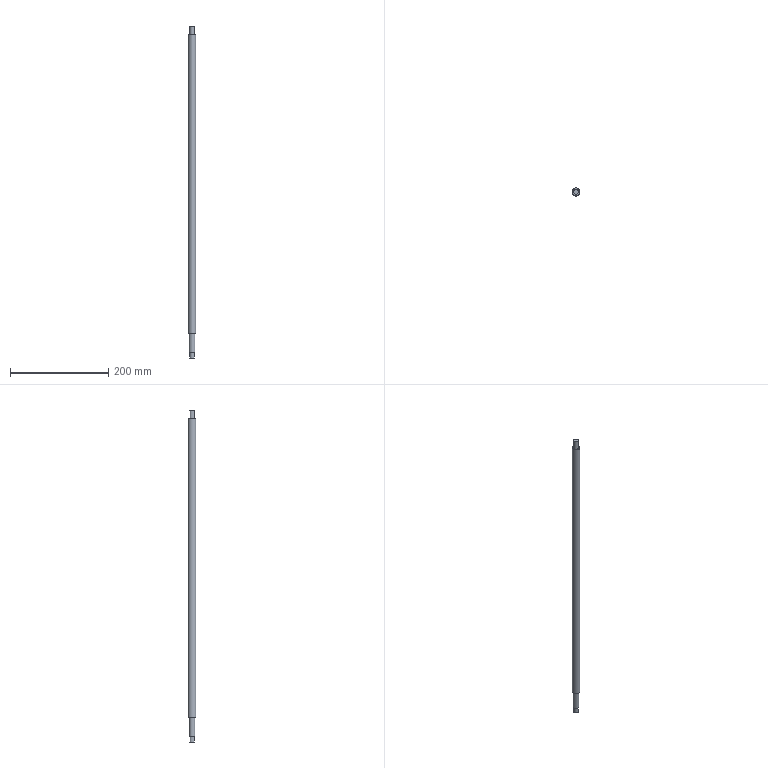Part | STEP file | 1 solid | 9 faces | box 16 x 16 x 675 mm | volume 128698 mm3 | plane 5 | cylinder 4 | commonest cylinder face diameters 10 x2 12 x1 16 x1
STEP:
#1=CARTESIAN_POINT('',(0.,0.,0.));
#2=DIRECTION('',(0.,0.,1.));
#3=DIRECTION('',(1.,0.,0.));
#4=AXIS2_PLACEMENT_3D('',#1,#2,#3);
#5=CARTESIAN_POINT('',(-8.,0.,0.));
#6=VERTEX_POINT('',#5);
#7=CARTESIAN_POINT('',(0.,0.,0.));
#8=DIRECTION('',(0.,0.,1.));
#9=DIRECTION('',(-1.,0.,0.));
#10=AXIS2_PLACEMENT_3D('',#7,#8,#9);
#11=CIRCLE('',#10,8.);
#12=CARTESIAN_POINT('',(0.,0.,607.));
#13=DIRECTION('',(0.,0.,-1.));
#14=DIRECTION('',(-1.,0.,0.));
#15=AXIS2_PLACEMENT_3D('',#12,#13,#14);
#16=CYLINDRICAL_SURFACE('',#15,8.);
#17=CARTESIAN_POINT('',(6.283,607.));
#18=DIRECTION('',(-1.,0.));
#19=VECTOR('',#18,1.);
#20=LINE('',#17,#19);
#21=(GEOMETRIC_REPRESENTATION_CONTEXT(2)PARAMETRIC_REPRESENTATION_CONTEXT()REPRESENTATION_CONTEXT('',''));
#22=DEFINITIONAL_REPRESENTATION('',(#20),#21);
#23=PCURVE('',#16,#22);
#24=CARTESIAN_POINT('',(0.,0.,0.));
#25=DIRECTION('',(0.,0.,1.));
#26=DIRECTION('',(1.,0.,0.));
#27=AXIS2_PLACEMENT_3D('',#24,#25,#26);
#28=PLANE('',#27);
#29=CARTESIAN_POINT('',(0.,0.));
#30=DIRECTION('',(-1.,0.));
#31=AXIS2_PLACEMENT_2D('',#29,#30);
#32=CIRCLE('',#31,8.);
#33=(GEOMETRIC_REPRESENTATION_CONTEXT(2)PARAMETRIC_REPRESENTATION_CONTEXT()REPRESENTATION_CONTEXT('',''));
#34=DEFINITIONAL_REPRESENTATION('',(#32),#33);
#35=PCURVE('',#28,#34);
#36=SURFACE_CURVE('',#11,(#23,#35),.PCURVE_S1.);
#37=EDGE_CURVE('',#6,#6,#36,.T.);
#38=ORIENTED_EDGE('',*,*,#37,.T.);
#39=CARTESIAN_POINT('',(-8.,0.,607.));
#40=VERTEX_POINT('',#39);
#41=CARTESIAN_POINT('',(-8.,0.,607.));
#42=CARTESIAN_POINT('',(-8.,0.,0.));
#43=B_SPLINE_CURVE_WITH_KNOTS('',1,(#41,#42),.UNSPECIFIED.,.F.,.F.,(2,2),(0.,607.),.PIECEWISE_BEZIER_KNOTS.);
#44=CARTESIAN_POINT('',(0.,0.));
#45=DIRECTION('',(0.,1.));
#46=VECTOR('',#45,1.);
#47=LINE('',#44,#46);
#48=(GEOMETRIC_REPRESENTATION_CONTEXT(2)PARAMETRIC_REPRESENTATION_CONTEXT()REPRESENTATION_CONTEXT('',''));
#49=DEFINITIONAL_REPRESENTATION('',(#47),#48);
#50=PCURVE('',#16,#49);
#51=CARTESIAN_POINT('',(6.283,0.));
#52=DIRECTION('',(0.,1.));
#53=VECTOR('',#52,1.);
#54=LINE('',#51,#53);
#55=(GEOMETRIC_REPRESENTATION_CONTEXT(2)PARAMETRIC_REPRESENTATION_CONTEXT()REPRESENTATION_CONTEXT('',''));
#56=DEFINITIONAL_REPRESENTATION('',(#54),#55);
#57=PCURVE('',#16,#56);
#58=SEAM_CURVE('',#43,(#50,#57),.PCURVE_S1.);
#59=EDGE_CURVE('',#40,#6,#58,.T.);
#60=ORIENTED_EDGE('',*,*,#59,.F.);
#61=CARTESIAN_POINT('',(0.,0.,607.));
#62=DIRECTION('',(0.,0.,-1.));
#63=DIRECTION('',(-1.,0.,0.));
#64=AXIS2_PLACEMENT_3D('',#61,#62,#63);
#65=CIRCLE('',#64,8.);
#66=CARTESIAN_POINT('',(0.,0.));
#67=DIRECTION('',(1.,0.));
#68=VECTOR('',#67,1.);
#69=LINE('',#66,#68);
#70=(GEOMETRIC_REPRESENTATION_CONTEXT(2)PARAMETRIC_REPRESENTATION_CONTEXT()REPRESENTATION_CONTEXT('',''));
#71=DEFINITIONAL_REPRESENTATION('',(#69),#70);
#72=PCURVE('',#16,#71);
#73=CARTESIAN_POINT('',(0.,0.,607.));
#74=DIRECTION('',(0.,0.,1.));
#75=DIRECTION('',(1.,0.,0.));
#76=AXIS2_PLACEMENT_3D('',#73,#74,#75);
#77=PLANE('',#76);
#78=CARTESIAN_POINT('',(-8.,0.));
#79=CARTESIAN_POINT('',(-8.,13.856));
#80=CARTESIAN_POINT('',(4.,6.928));
#81=CARTESIAN_POINT('',(16.,0.));
#82=CARTESIAN_POINT('',(4.,-6.928));
#83=CARTESIAN_POINT('',(-8.,-13.856));
#84=CARTESIAN_POINT('',(-8.,0.));
#85=(BOUNDED_CURVE()B_SPLINE_CURVE(2,(#78,#79,#80,#81,#82,#83,#84),.UNSPECIFIED.,.T.,.F.)B_SPLINE_CURVE_WITH_KNOTS((1,2,2,2,2,1),(-2.094,0.,2.094,4.189,6.283,8.378),.UNSPECIFIED.)CURVE()GEOMETRIC_REPRESENTATION_ITEM()RATIONAL_B_SPLINE_CURVE((1.,0.5,1.,0.5,1.,0.5,1.))REPRESENTATION_ITEM(''));
#86=(GEOMETRIC_REPRESENTATION_CONTEXT(2)PARAMETRIC_REPRESENTATION_CONTEXT()REPRESENTATION_CONTEXT('',''));
#87=DEFINITIONAL_REPRESENTATION('',(#85),#86);
#88=PCURVE('',#77,#87);
#89=SURFACE_CURVE('',#65,(#72,#88),.PCURVE_S1.);
#90=EDGE_CURVE('',#40,#40,#89,.T.);
#91=ORIENTED_EDGE('',*,*,#90,.T.);
#92=ORIENTED_EDGE('',*,*,#59,.T.);
#93=EDGE_LOOP('',(#38,#60,#91,#92));
#94=FACE_BOUND('',#93,.T.);
#95=ADVANCED_FACE('',(#94),#16,.T.);
#96=CARTESIAN_POINT('',(6.,0.,0.));
#97=VERTEX_POINT('',#96);
#98=CARTESIAN_POINT('',(0.,0.,0.));
#99=DIRECTION('',(0.,0.,-1.));
#100=DIRECTION('',(1.,0.,0.));
#101=AXIS2_PLACEMENT_3D('',#98,#99,#100);
#102=CIRCLE('',#101,6.);
#103=CARTESIAN_POINT('',(6.,0.));
#104=CARTESIAN_POINT('',(6.,-10.392));
#105=CARTESIAN_POINT('',(-3.,-5.196));
#106=CARTESIAN_POINT('',(-12.,0.));
#107=CARTESIAN_POINT('',(-3.,5.196));
#108=CARTESIAN_POINT('',(6.,10.392));
#109=CARTESIAN_POINT('',(6.,0.));
#110=(BOUNDED_CURVE()B_SPLINE_CURVE(2,(#103,#104,#105,#106,#107,#108,#109),.UNSPECIFIED.,.T.,.F.)B_SPLINE_CURVE_WITH_KNOTS((1,2,2,2,2,1),(-2.094,0.,2.094,4.189,6.283,8.378),.UNSPECIFIED.)CURVE()GEOMETRIC_REPRESENTATION_ITEM()RATIONAL_B_SPLINE_CURVE((1.,0.5,1.,0.5,1.,0.5,1.))REPRESENTATION_ITEM(''));
#111=(GEOMETRIC_REPRESENTATION_CONTEXT(2)PARAMETRIC_REPRESENTATION_CONTEXT()REPRESENTATION_CONTEXT('',''));
#112=DEFINITIONAL_REPRESENTATION('',(#110),#111);
#113=PCURVE('',#28,#112);
#114=CARTESIAN_POINT('',(0.,0.,-38.));
#115=DIRECTION('',(0.,0.,1.));
#116=DIRECTION('',(1.,0.,0.));
#117=AXIS2_PLACEMENT_3D('',#114,#115,#116);
#118=CYLINDRICAL_SURFACE('',#117,6.);
#119=CARTESIAN_POINT('',(6.283,38.));
#120=DIRECTION('',(-1.,0.));
#121=VECTOR('',#120,1.);
#122=LINE('',#119,#121);
#123=(GEOMETRIC_REPRESENTATION_CONTEXT(2)PARAMETRIC_REPRESENTATION_CONTEXT()REPRESENTATION_CONTEXT('',''));
#124=DEFINITIONAL_REPRESENTATION('',(#122),#123);
#125=PCURVE('',#118,#124);
#126=SURFACE_CURVE('',#102,(#113,#125),.PCURVE_S1.);
#127=EDGE_CURVE('',#97,#97,#126,.T.);
#128=ORIENTED_EDGE('',*,*,#127,.F.);
#129=EDGE_LOOP('',(#128));
#130=FACE_BOUND('',#129,.T.);
#131=ORIENTED_EDGE('',*,*,#37,.F.);
#132=EDGE_LOOP('',(#131));
#133=FACE_BOUND('',#132,.T.);
#134=ADVANCED_FACE('',(#130,#133),#28,.F.);
#135=CARTESIAN_POINT('',(-5.,0.,607.));
#136=VERTEX_POINT('',#135);
#137=CARTESIAN_POINT('',(0.,0.,607.));
#138=DIRECTION('',(0.,0.,-1.));
#139=DIRECTION('',(-1.,0.,0.));
#140=AXIS2_PLACEMENT_3D('',#137,#138,#139);
#141=CIRCLE('',#140,5.);
#142=CARTESIAN_POINT('',(-5.,0.));
#143=CARTESIAN_POINT('',(-5.,8.66));
#144=CARTESIAN_POINT('',(2.5,4.33));
#145=CARTESIAN_POINT('',(10.,0.));
#146=CARTESIAN_POINT('',(2.5,-4.33));
#147=CARTESIAN_POINT('',(-5.,-8.66));
#148=CARTESIAN_POINT('',(-5.,0.));
#149=(BOUNDED_CURVE()B_SPLINE_CURVE(2,(#142,#143,#144,#145,#146,#147,#148),.UNSPECIFIED.,.T.,.F.)B_SPLINE_CURVE_WITH_KNOTS((1,2,2,2,2,1),(-2.094,0.,2.094,4.189,6.283,8.378),.UNSPECIFIED.)CURVE()GEOMETRIC_REPRESENTATION_ITEM()RATIONAL_B_SPLINE_CURVE((1.,0.5,1.,0.5,1.,0.5,1.))REPRESENTATION_ITEM(''));
#150=(GEOMETRIC_REPRESENTATION_CONTEXT(2)PARAMETRIC_REPRESENTATION_CONTEXT()REPRESENTATION_CONTEXT('',''));
#151=DEFINITIONAL_REPRESENTATION('',(#149),#150);
#152=PCURVE('',#77,#151);
#153=CARTESIAN_POINT('',(0.,0.,625.));
#154=DIRECTION('',(0.,0.,-1.));
#155=DIRECTION('',(-1.,0.,0.));
#156=AXIS2_PLACEMENT_3D('',#153,#154,#155);
#157=CYLINDRICAL_SURFACE('',#156,5.);
#158=CARTESIAN_POINT('',(0.,18.));
#159=DIRECTION('',(1.,0.));
#160=VECTOR('',#159,1.);
#161=LINE('',#158,#160);
#162=(GEOMETRIC_REPRESENTATION_CONTEXT(2)PARAMETRIC_REPRESENTATION_CONTEXT()REPRESENTATION_CONTEXT('',''));
#163=DEFINITIONAL_REPRESENTATION('',(#161),#162);
#164=PCURVE('',#157,#163);
#165=SURFACE_CURVE('',#141,(#152,#164),.PCURVE_S1.);
#166=EDGE_CURVE('',#136,#136,#165,.T.);
#167=ORIENTED_EDGE('',*,*,#166,.T.);
#168=EDGE_LOOP('',(#167));
#169=FACE_BOUND('',#168,.T.);
#170=ORIENTED_EDGE('',*,*,#90,.F.);
#171=EDGE_LOOP('',(#170));
#172=FACE_BOUND('',#171,.T.);
#173=ADVANCED_FACE('',(#169,#172),#77,.T.);
#174=CARTESIAN_POINT('',(6.,0.,-38.));
#175=VERTEX_POINT('',#174);
#176=CARTESIAN_POINT('',(0.,0.,-38.));
#177=DIRECTION('',(0.,0.,1.));
#178=DIRECTION('',(1.,0.,0.));
#179=AXIS2_PLACEMENT_3D('',#176,#177,#178);
#180=CIRCLE('',#179,6.);
#181=CARTESIAN_POINT('',(0.,0.));
#182=DIRECTION('',(1.,0.));
#183=VECTOR('',#182,1.);
#184=LINE('',#181,#183);
#185=(GEOMETRIC_REPRESENTATION_CONTEXT(2)PARAMETRIC_REPRESENTATION_CONTEXT()REPRESENTATION_CONTEXT('',''));
#186=DEFINITIONAL_REPRESENTATION('',(#184),#185);
#187=PCURVE('',#118,#186);
#188=CARTESIAN_POINT('',(0.,0.,-38.));
#189=DIRECTION('',(0.,0.,-1.));
#190=DIRECTION('',(-1.,0.,0.));
#191=AXIS2_PLACEMENT_3D('',#188,#189,#190);
#192=PLANE('',#191);
#193=CARTESIAN_POINT('',(-6.,0.));
#194=CARTESIAN_POINT('',(-6.,10.392));
#195=CARTESIAN_POINT('',(3.,5.196));
#196=CARTESIAN_POINT('',(12.,0.));
#197=CARTESIAN_POINT('',(3.,-5.196));
#198=CARTESIAN_POINT('',(-6.,-10.392));
#199=CARTESIAN_POINT('',(-6.,0.));
#200=(BOUNDED_CURVE()B_SPLINE_CURVE(2,(#193,#194,#195,#196,#197,#198,#199),.UNSPECIFIED.,.T.,.F.)B_SPLINE_CURVE_WITH_KNOTS((1,2,2,2,2,1),(-2.094,0.,2.094,4.189,6.283,8.378),.UNSPECIFIED.)CURVE()GEOMETRIC_REPRESENTATION_ITEM()RATIONAL_B_SPLINE_CURVE((1.,0.5,1.,0.5,1.,0.5,1.))REPRESENTATION_ITEM(''));
#201=(GEOMETRIC_REPRESENTATION_CONTEXT(2)PARAMETRIC_REPRESENTATION_CONTEXT()REPRESENTATION_CONTEXT('',''));
#202=DEFINITIONAL_REPRESENTATION('',(#200),#201);
#203=PCURVE('',#192,#202);
#204=SURFACE_CURVE('',#180,(#187,#203),.PCURVE_S1.);
#205=EDGE_CURVE('',#175,#175,#204,.T.);
#206=ORIENTED_EDGE('',*,*,#205,.T.);
#207=CARTESIAN_POINT('',(6.,0.,-38.));
#208=CARTESIAN_POINT('',(6.,0.,0.));
#209=B_SPLINE_CURVE_WITH_KNOTS('',1,(#207,#208),.UNSPECIFIED.,.F.,.F.,(2,2),(0.,38.),.PIECEWISE_BEZIER_KNOTS.);
#210=CARTESIAN_POINT('',(6.283,0.));
#211=DIRECTION('',(0.,1.));
#212=VECTOR('',#211,1.);
#213=LINE('',#210,#212);
#214=(GEOMETRIC_REPRESENTATION_CONTEXT(2)PARAMETRIC_REPRESENTATION_CONTEXT()REPRESENTATION_CONTEXT('',''));
#215=DEFINITIONAL_REPRESENTATION('',(#213),#214);
#216=PCURVE('',#118,#215);
#217=CARTESIAN_POINT('',(0.,0.));
#218=DIRECTION('',(0.,1.));
#219=VECTOR('',#218,1.);
#220=LINE('',#217,#219);
#221=(GEOMETRIC_REPRESENTATION_CONTEXT(2)PARAMETRIC_REPRESENTATION_CONTEXT()REPRESENTATION_CONTEXT('',''));
#222=DEFINITIONAL_REPRESENTATION('',(#220),#221);
#223=PCURVE('',#118,#222);
#224=SEAM_CURVE('',#209,(#216,#223),.PCURVE_S1.);
#225=EDGE_CURVE('',#175,#97,#224,.T.);
#226=ORIENTED_EDGE('',*,*,#225,.T.);
#227=ORIENTED_EDGE('',*,*,#127,.T.);
#228=ORIENTED_EDGE('',*,*,#225,.F.);
#229=EDGE_LOOP('',(#206,#226,#227,#228));
#230=FACE_BOUND('',#229,.T.);
#231=ADVANCED_FACE('',(#230),#118,.T.);
#232=ORIENTED_EDGE('',*,*,#166,.F.);
#233=CARTESIAN_POINT('',(-5.,0.,625.));
#234=VERTEX_POINT('',#233);
#235=CARTESIAN_POINT('',(-5.,0.,625.));
#236=CARTESIAN_POINT('',(-5.,0.,607.));
#237=B_SPLINE_CURVE_WITH_KNOTS('',1,(#235,#236),.UNSPECIFIED.,.F.,.F.,(2,2),(0.,18.),.PIECEWISE_BEZIER_KNOTS.);
#238=CARTESIAN_POINT('',(0.,0.));
#239=DIRECTION('',(0.,1.));
#240=VECTOR('',#239,1.);
#241=LINE('',#238,#240);
#242=(GEOMETRIC_REPRESENTATION_CONTEXT(2)PARAMETRIC_REPRESENTATION_CONTEXT()REPRESENTATION_CONTEXT('',''));
#243=DEFINITIONAL_REPRESENTATION('',(#241),#242);
#244=PCURVE('',#157,#243);
#245=CARTESIAN_POINT('',(6.283,0.));
#246=DIRECTION('',(0.,1.));
#247=VECTOR('',#246,1.);
#248=LINE('',#245,#247);
#249=(GEOMETRIC_REPRESENTATION_CONTEXT(2)PARAMETRIC_REPRESENTATION_CONTEXT()REPRESENTATION_CONTEXT('',''));
#250=DEFINITIONAL_REPRESENTATION('',(#248),#249);
#251=PCURVE('',#157,#250);
#252=SEAM_CURVE('',#237,(#244,#251),.PCURVE_S1.);
#253=EDGE_CURVE('',#234,#136,#252,.T.);
#254=ORIENTED_EDGE('',*,*,#253,.F.);
#255=CARTESIAN_POINT('',(0.,0.,625.));
#256=DIRECTION('',(0.,0.,-1.));
#257=DIRECTION('',(-1.,0.,0.));
#258=AXIS2_PLACEMENT_3D('',#255,#256,#257);
#259=CIRCLE('',#258,5.);
#260=CARTESIAN_POINT('',(0.,0.));
#261=DIRECTION('',(1.,0.));
#262=VECTOR('',#261,1.);
#263=LINE('',#260,#262);
#264=(GEOMETRIC_REPRESENTATION_CONTEXT(2)PARAMETRIC_REPRESENTATION_CONTEXT()REPRESENTATION_CONTEXT('',''));
#265=DEFINITIONAL_REPRESENTATION('',(#263),#264);
#266=PCURVE('',#157,#265);
#267=CARTESIAN_POINT('',(0.,0.,625.));
#268=DIRECTION('',(0.,0.,1.));
#269=DIRECTION('',(1.,0.,0.));
#270=AXIS2_PLACEMENT_3D('',#267,#268,#269);
#271=PLANE('',#270);
#272=CARTESIAN_POINT('',(-5.,0.));
#273=CARTESIAN_POINT('',(-5.,8.66));
#274=CARTESIAN_POINT('',(2.5,4.33));
#275=CARTESIAN_POINT('',(10.,0.));
#276=CARTESIAN_POINT('',(2.5,-4.33));
#277=CARTESIAN_POINT('',(-5.,-8.66));
#278=CARTESIAN_POINT('',(-5.,0.));
#279=(BOUNDED_CURVE()B_SPLINE_CURVE(2,(#272,#273,#274,#275,#276,#277,#278),.UNSPECIFIED.,.T.,.F.)B_SPLINE_CURVE_WITH_KNOTS((1,2,2,2,2,1),(-2.094,0.,2.094,4.189,6.283,8.378),.UNSPECIFIED.)CURVE()GEOMETRIC_REPRESENTATION_ITEM()RATIONAL_B_SPLINE_CURVE((1.,0.5,1.,0.5,1.,0.5,1.))REPRESENTATION_ITEM(''));
#280=(GEOMETRIC_REPRESENTATION_CONTEXT(2)PARAMETRIC_REPRESENTATION_CONTEXT()REPRESENTATION_CONTEXT('',''));
#281=DEFINITIONAL_REPRESENTATION('',(#279),#280);
#282=PCURVE('',#271,#281);
#283=SURFACE_CURVE('',#259,(#266,#282),.PCURVE_S1.);
#284=EDGE_CURVE('',#234,#234,#283,.T.);
#285=ORIENTED_EDGE('',*,*,#284,.T.);
#286=ORIENTED_EDGE('',*,*,#253,.T.);
#287=EDGE_LOOP('',(#232,#254,#285,#286));
#288=FACE_BOUND('',#287,.T.);
#289=ADVANCED_FACE('',(#288),#157,.T.);
#290=CARTESIAN_POINT('',(5.,0.,-38.));
#291=VERTEX_POINT('',#290);
#292=CARTESIAN_POINT('',(0.,0.,-38.));
#293=DIRECTION('',(0.,0.,1.));
#294=DIRECTION('',(1.,0.,0.));
#295=AXIS2_PLACEMENT_3D('',#292,#293,#294);
#296=CIRCLE('',#295,5.);
#297=CARTESIAN_POINT('',(-5.,0.));
#298=CARTESIAN_POINT('',(-5.,8.66));
#299=CARTESIAN_POINT('',(2.5,4.33));
#300=CARTESIAN_POINT('',(10.,0.));
#301=CARTESIAN_POINT('',(2.5,-4.33));
#302=CARTESIAN_POINT('',(-5.,-8.66));
#303=CARTESIAN_POINT('',(-5.,0.));
#304=(BOUNDED_CURVE()B_SPLINE_CURVE(2,(#297,#298,#299,#300,#301,#302,#303),.UNSPECIFIED.,.T.,.F.)B_SPLINE_CURVE_WITH_KNOTS((1,2,2,2,2,1),(-2.094,0.,2.094,4.189,6.283,8.378),.UNSPECIFIED.)CURVE()GEOMETRIC_REPRESENTATION_ITEM()RATIONAL_B_SPLINE_CURVE((1.,0.5,1.,0.5,1.,0.5,1.))REPRESENTATION_ITEM(''));
#305=(GEOMETRIC_REPRESENTATION_CONTEXT(2)PARAMETRIC_REPRESENTATION_CONTEXT()REPRESENTATION_CONTEXT('',''));
#306=DEFINITIONAL_REPRESENTATION('',(#304),#305);
#307=PCURVE('',#192,#306);
#308=CARTESIAN_POINT('',(0.,0.,-50.));
#309=DIRECTION('',(0.,0.,1.));
#310=DIRECTION('',(1.,0.,0.));
#311=AXIS2_PLACEMENT_3D('',#308,#309,#310);
#312=CYLINDRICAL_SURFACE('',#311,5.);
#313=CARTESIAN_POINT('',(0.,12.));
#314=DIRECTION('',(1.,0.));
#315=VECTOR('',#314,1.);
#316=LINE('',#313,#315);
#317=(GEOMETRIC_REPRESENTATION_CONTEXT(2)PARAMETRIC_REPRESENTATION_CONTEXT()REPRESENTATION_CONTEXT('',''));
#318=DEFINITIONAL_REPRESENTATION('',(#316),#317);
#319=PCURVE('',#312,#318);
#320=SURFACE_CURVE('',#296,(#307,#319),.PCURVE_S1.);
#321=EDGE_CURVE('',#291,#291,#320,.T.);
#322=ORIENTED_EDGE('',*,*,#321,.T.);
#323=EDGE_LOOP('',(#322));
#324=FACE_BOUND('',#323,.T.);
#325=ORIENTED_EDGE('',*,*,#205,.F.);
#326=EDGE_LOOP('',(#325));
#327=FACE_BOUND('',#326,.T.);
#328=ADVANCED_FACE('',(#324,#327),#192,.T.);
#329=ORIENTED_EDGE('',*,*,#284,.F.);
#330=EDGE_LOOP('',(#329));
#331=FACE_BOUND('',#330,.T.);
#332=ADVANCED_FACE('',(#331),#271,.T.);
#333=ORIENTED_EDGE('',*,*,#321,.F.);
#334=CARTESIAN_POINT('',(5.,0.,-50.));
#335=VERTEX_POINT('',#334);
#336=CARTESIAN_POINT('',(5.,0.,-50.));
#337=CARTESIAN_POINT('',(5.,0.,-38.));
#338=B_SPLINE_CURVE_WITH_KNOTS('',1,(#336,#337),.UNSPECIFIED.,.F.,.F.,(2,2),(0.,12.),.PIECEWISE_BEZIER_KNOTS.);
#339=CARTESIAN_POINT('',(0.,0.));
#340=DIRECTION('',(0.,1.));
#341=VECTOR('',#340,1.);
#342=LINE('',#339,#341);
#343=(GEOMETRIC_REPRESENTATION_CONTEXT(2)PARAMETRIC_REPRESENTATION_CONTEXT()REPRESENTATION_CONTEXT('',''));
#344=DEFINITIONAL_REPRESENTATION('',(#342),#343);
#345=PCURVE('',#312,#344);
#346=CARTESIAN_POINT('',(6.283,0.));
#347=DIRECTION('',(0.,1.));
#348=VECTOR('',#347,1.);
#349=LINE('',#346,#348);
#350=(GEOMETRIC_REPRESENTATION_CONTEXT(2)PARAMETRIC_REPRESENTATION_CONTEXT()REPRESENTATION_CONTEXT('',''));
#351=DEFINITIONAL_REPRESENTATION('',(#349),#350);
#352=PCURVE('',#312,#351);
#353=SEAM_CURVE('',#338,(#345,#352),.PCURVE_S1.);
#354=EDGE_CURVE('',#335,#291,#353,.T.);
#355=ORIENTED_EDGE('',*,*,#354,.F.);
#356=CARTESIAN_POINT('',(0.,0.,-50.));
#357=DIRECTION('',(0.,0.,1.));
#358=DIRECTION('',(1.,0.,0.));
#359=AXIS2_PLACEMENT_3D('',#356,#357,#358);
#360=CIRCLE('',#359,5.);
#361=CARTESIAN_POINT('',(0.,0.));
#362=DIRECTION('',(1.,0.));
#363=VECTOR('',#362,1.);
#364=LINE('',#361,#363);
#365=(GEOMETRIC_REPRESENTATION_CONTEXT(2)PARAMETRIC_REPRESENTATION_CONTEXT()REPRESENTATION_CONTEXT('',''));
#366=DEFINITIONAL_REPRESENTATION('',(#364),#365);
#367=PCURVE('',#312,#366);
#368=CARTESIAN_POINT('',(0.,0.,-50.));
#369=DIRECTION('',(0.,0.,-1.));
#370=DIRECTION('',(-1.,0.,0.));
#371=AXIS2_PLACEMENT_3D('',#368,#369,#370);
#372=PLANE('',#371);
#373=CARTESIAN_POINT('',(-5.,0.));
#374=CARTESIAN_POINT('',(-5.,8.66));
#375=CARTESIAN_POINT('',(2.5,4.33));
#376=CARTESIAN_POINT('',(10.,0.));
#377=CARTESIAN_POINT('',(2.5,-4.33));
#378=CARTESIAN_POINT('',(-5.,-8.66));
#379=CARTESIAN_POINT('',(-5.,0.));
#380=(BOUNDED_CURVE()B_SPLINE_CURVE(2,(#373,#374,#375,#376,#377,#378,#379),.UNSPECIFIED.,.T.,.F.)B_SPLINE_CURVE_WITH_KNOTS((1,2,2,2,2,1),(-2.094,0.,2.094,4.189,6.283,8.378),.UNSPECIFIED.)CURVE()GEOMETRIC_REPRESENTATION_ITEM()RATIONAL_B_SPLINE_CURVE((1.,0.5,1.,0.5,1.,0.5,1.))REPRESENTATION_ITEM(''));
#381=(GEOMETRIC_REPRESENTATION_CONTEXT(2)PARAMETRIC_REPRESENTATION_CONTEXT()REPRESENTATION_CONTEXT('',''));
#382=DEFINITIONAL_REPRESENTATION('',(#380),#381);
#383=PCURVE('',#372,#382);
#384=SURFACE_CURVE('',#360,(#367,#383),.PCURVE_S1.);
#385=EDGE_CURVE('',#335,#335,#384,.T.);
#386=ORIENTED_EDGE('',*,*,#385,.T.);
#387=ORIENTED_EDGE('',*,*,#354,.T.);
#388=EDGE_LOOP('',(#333,#355,#386,#387));
#389=FACE_BOUND('',#388,.T.);
#390=ADVANCED_FACE('',(#389),#312,.T.);
#391=ORIENTED_EDGE('',*,*,#385,.F.);
#392=EDGE_LOOP('',(#391));
#393=FACE_BOUND('',#392,.T.);
#394=ADVANCED_FACE('',(#393),#372,.T.);
#395=CLOSED_SHELL('',(#95,#134,#173,#231,#289,#328,#332,#390,#394));
#396=MANIFOLD_SOLID_BREP('',#395);
#397=(LENGTH_UNIT()NAMED_UNIT(*)SI_UNIT(.MILLI.,.METRE.));
#398=UNCERTAINTY_MEASURE_WITH_UNIT(LENGTH_MEASURE(0.00001),#397,'','');
#399=(NAMED_UNIT(*)PLANE_ANGLE_UNIT()SI_UNIT($,.RADIAN.));
#400=(NAMED_UNIT(*)SI_UNIT($,.STERADIAN.)SOLID_ANGLE_UNIT());
#401=(GEOMETRIC_REPRESENTATION_CONTEXT(3)GLOBAL_UNCERTAINTY_ASSIGNED_CONTEXT((#398))GLOBAL_UNIT_ASSIGNED_CONTEXT((#397,#399,#400))REPRESENTATION_CONTEXT('',''));
#402=ADVANCED_BREP_SHAPE_REPRESENTATION('',(#4,#396),#401);